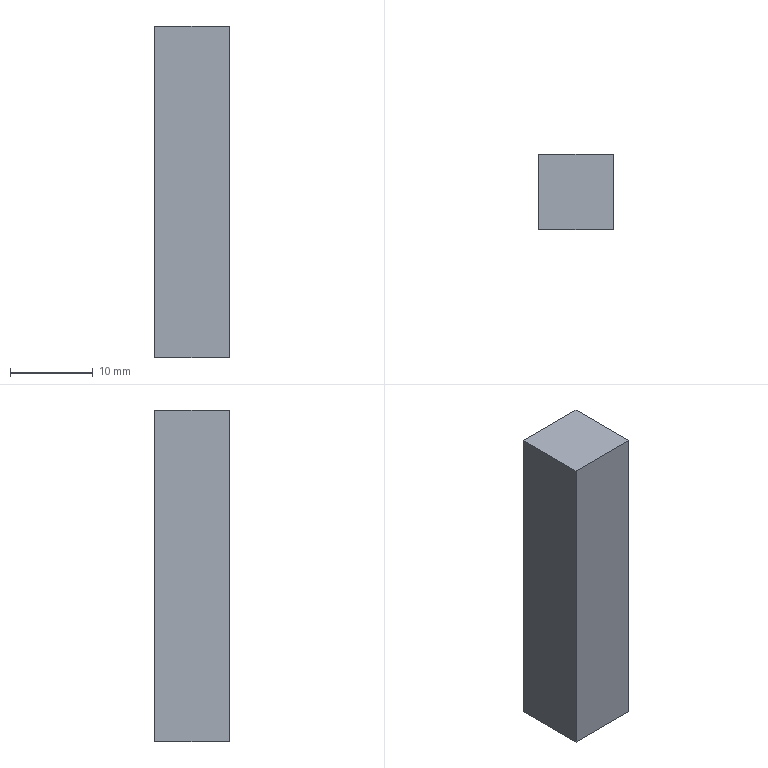Part | SolidWorks | features FlatPattern 1, SMBaseFlange 1, SheetMetal 1 | 1 solid | 6 faces | box 9 x 9 x 40 mm | volume 3240 mm3 | plane 6
STEP:
#1=CARTESIAN_POINT('',(0.,-9.,0.));
#2=VERTEX_POINT('',#1);
#3=CARTESIAN_POINT('',(0.,-9.,-40.));
#4=VERTEX_POINT('',#3);
#5=CARTESIAN_POINT('',(0.,-9.,0.));
#6=DIRECTION('',(0.,0.,-1.));
#7=VECTOR('',#6,1000.);
#8=LINE('',#5,#7);
#9=EDGE_CURVE('',#2,#4,#8,.T.);
#10=ORIENTED_EDGE('',*,*,#9,.T.);
#11=CARTESIAN_POINT('',(9.,-9.,-40.));
#12=VERTEX_POINT('',#11);
#13=CARTESIAN_POINT('',(9.,-9.,-40.));
#14=DIRECTION('',(-1.,0.,0.));
#15=VECTOR('',#14,1000.);
#16=LINE('',#13,#15);
#17=EDGE_CURVE('',#12,#4,#16,.T.);
#18=ORIENTED_EDGE('',*,*,#17,.F.);
#19=CARTESIAN_POINT('',(9.,-9.,0.));
#20=VERTEX_POINT('',#19);
#21=CARTESIAN_POINT('',(9.,-9.,0.));
#22=DIRECTION('',(0.,0.,-1.));
#23=VECTOR('',#22,1000.);
#24=LINE('',#21,#23);
#25=EDGE_CURVE('',#20,#12,#24,.T.);
#26=ORIENTED_EDGE('',*,*,#25,.F.);
#27=CARTESIAN_POINT('',(9.,-9.,0.));
#28=DIRECTION('',(-1.,0.,0.));
#29=VECTOR('',#28,1000.);
#30=LINE('',#27,#29);
#31=EDGE_CURVE('',#20,#2,#30,.T.);
#32=ORIENTED_EDGE('',*,*,#31,.T.);
#33=EDGE_LOOP('',(#10,#18,#26,#32));
#34=FACE_OUTER_BOUND('',#33,.T.);
#35=CARTESIAN_POINT('',(9.,-9.,0.));
#36=DIRECTION('',(0.,1.,0.));
#37=DIRECTION('',(0.,0.,1.));
#38=AXIS2_PLACEMENT_3D('',#35,#36,#37);
#39=PLANE('',#38);
#40=ADVANCED_FACE('',(#34),#39,.F.);
#41=CARTESIAN_POINT('',(0.,0.,-40.));
#42=VERTEX_POINT('',#41);
#43=CARTESIAN_POINT('',(0.,0.,-40.));
#44=DIRECTION('',(0.,-1.,0.));
#45=VECTOR('',#44,1000.);
#46=LINE('',#43,#45);
#47=EDGE_CURVE('',#42,#4,#46,.T.);
#48=ORIENTED_EDGE('',*,*,#47,.F.);
#49=CARTESIAN_POINT('',(9.,0.,-40.));
#50=VERTEX_POINT('',#49);
#51=CARTESIAN_POINT('',(9.,0.,-40.));
#52=DIRECTION('',(-1.,0.,0.));
#53=VECTOR('',#52,1000.);
#54=LINE('',#51,#53);
#55=EDGE_CURVE('',#50,#42,#54,.T.);
#56=ORIENTED_EDGE('',*,*,#55,.F.);
#57=CARTESIAN_POINT('',(9.,0.,-40.));
#58=DIRECTION('',(0.,-1.,0.));
#59=VECTOR('',#58,1000.);
#60=LINE('',#57,#59);
#61=EDGE_CURVE('',#50,#12,#60,.T.);
#62=ORIENTED_EDGE('',*,*,#61,.T.);
#63=ORIENTED_EDGE('',*,*,#17,.T.);
#64=EDGE_LOOP('',(#48,#56,#62,#63));
#65=FACE_OUTER_BOUND('',#64,.T.);
#66=CARTESIAN_POINT('',(9.,0.,-40.));
#67=DIRECTION('',(0.,0.,-1.));
#68=DIRECTION('',(-1.,0.,0.));
#69=AXIS2_PLACEMENT_3D('',#66,#67,#68);
#70=PLANE('',#69);
#71=ADVANCED_FACE('',(#65),#70,.T.);
#72=CARTESIAN_POINT('',(0.,0.,0.));
#73=VERTEX_POINT('',#72);
#74=CARTESIAN_POINT('',(0.,0.,0.));
#75=DIRECTION('',(0.,0.,-1.));
#76=VECTOR('',#75,1000.);
#77=LINE('',#74,#76);
#78=EDGE_CURVE('',#73,#42,#77,.T.);
#79=ORIENTED_EDGE('',*,*,#78,.F.);
#80=CARTESIAN_POINT('',(9.,0.,0.));
#81=VERTEX_POINT('',#80);
#82=CARTESIAN_POINT('',(9.,0.,0.));
#83=DIRECTION('',(-1.,0.,0.));
#84=VECTOR('',#83,1000.);
#85=LINE('',#82,#84);
#86=EDGE_CURVE('',#81,#73,#85,.T.);
#87=ORIENTED_EDGE('',*,*,#86,.F.);
#88=CARTESIAN_POINT('',(9.,0.,0.));
#89=DIRECTION('',(0.,0.,-1.));
#90=VECTOR('',#89,1000.);
#91=LINE('',#88,#90);
#92=EDGE_CURVE('',#81,#50,#91,.T.);
#93=ORIENTED_EDGE('',*,*,#92,.T.);
#94=ORIENTED_EDGE('',*,*,#55,.T.);
#95=EDGE_LOOP('',(#79,#87,#93,#94));
#96=FACE_OUTER_BOUND('',#95,.T.);
#97=CARTESIAN_POINT('',(9.,0.,0.));
#98=DIRECTION('',(0.,1.,0.));
#99=DIRECTION('',(0.,0.,1.));
#100=AXIS2_PLACEMENT_3D('',#97,#98,#99);
#101=PLANE('',#100);
#102=ADVANCED_FACE('',(#96),#101,.T.);
#103=CARTESIAN_POINT('',(0.,-9.,0.));
#104=DIRECTION('',(0.,1.,0.));
#105=VECTOR('',#104,1000.);
#106=LINE('',#103,#105);
#107=EDGE_CURVE('',#2,#73,#106,.T.);
#108=ORIENTED_EDGE('',*,*,#107,.F.);
#109=ORIENTED_EDGE('',*,*,#31,.F.);
#110=CARTESIAN_POINT('',(9.,-9.,0.));
#111=DIRECTION('',(0.,1.,0.));
#112=VECTOR('',#111,1000.);
#113=LINE('',#110,#112);
#114=EDGE_CURVE('',#20,#81,#113,.T.);
#115=ORIENTED_EDGE('',*,*,#114,.T.);
#116=ORIENTED_EDGE('',*,*,#86,.T.);
#117=EDGE_LOOP('',(#108,#109,#115,#116));
#118=FACE_OUTER_BOUND('',#117,.T.);
#119=CARTESIAN_POINT('',(9.,-9.,0.));
#120=DIRECTION('',(0.,0.,1.));
#121=DIRECTION('',(1.,0.,0.));
#122=AXIS2_PLACEMENT_3D('',#119,#120,#121);
#123=PLANE('',#122);
#124=ADVANCED_FACE('',(#118),#123,.T.);
#125=ORIENTED_EDGE('',*,*,#25,.T.);
#126=ORIENTED_EDGE('',*,*,#61,.F.);
#127=ORIENTED_EDGE('',*,*,#92,.F.);
#128=ORIENTED_EDGE('',*,*,#114,.F.);
#129=EDGE_LOOP('',(#125,#126,#127,#128));
#130=FACE_OUTER_BOUND('',#129,.T.);
#131=CARTESIAN_POINT('',(9.,0.,0.));
#132=DIRECTION('',(-1.,0.,0.));
#133=DIRECTION('',(0.,0.,1.));
#134=AXIS2_PLACEMENT_3D('',#131,#132,#133);
#135=PLANE('',#134);
#136=ADVANCED_FACE('',(#130),#135,.F.);
#137=ORIENTED_EDGE('',*,*,#9,.F.);
#138=ORIENTED_EDGE('',*,*,#107,.T.);
#139=ORIENTED_EDGE('',*,*,#78,.T.);
#140=ORIENTED_EDGE('',*,*,#47,.T.);
#141=EDGE_LOOP('',(#137,#138,#139,#140));
#142=FACE_OUTER_BOUND('',#141,.T.);
#143=CARTESIAN_POINT('',(0.,0.,0.));
#144=DIRECTION('',(-1.,0.,0.));
#145=DIRECTION('',(0.,0.,1.));
#146=AXIS2_PLACEMENT_3D('',#143,#144,#145);
#147=PLANE('',#146);
#148=ADVANCED_FACE('',(#142),#147,.T.);
#149=CLOSED_SHELL('',(#40,#71,#102,#124,#136,#148));
#150=MANIFOLD_SOLID_BREP('',#149);
#151=CARTESIAN_POINT('',(0.,0.,0.));
#152=DIRECTION('',(0.,0.,1.));
#153=DIRECTION('',(1.,0.,0.));
#154=AXIS2_PLACEMENT_3D('',#151,#152,#153);
#155=(LENGTH_UNIT()NAMED_UNIT(*)SI_UNIT(.MILLI.,.METRE.));
#156=UNCERTAINTY_MEASURE_WITH_UNIT(LENGTH_MEASURE(0.00001),#155,'','');
#157=(NAMED_UNIT(*)PLANE_ANGLE_UNIT()SI_UNIT($,.RADIAN.));
#158=(NAMED_UNIT(*)SI_UNIT($,.STERADIAN.)SOLID_ANGLE_UNIT());
#159=(GEOMETRIC_REPRESENTATION_CONTEXT(3)GLOBAL_UNCERTAINTY_ASSIGNED_CONTEXT((#156))GLOBAL_UNIT_ASSIGNED_CONTEXT((#155,#157,#158))REPRESENTATION_CONTEXT('',''));
#160=ADVANCED_BREP_SHAPE_REPRESENTATION('',(#150,#154),#159);